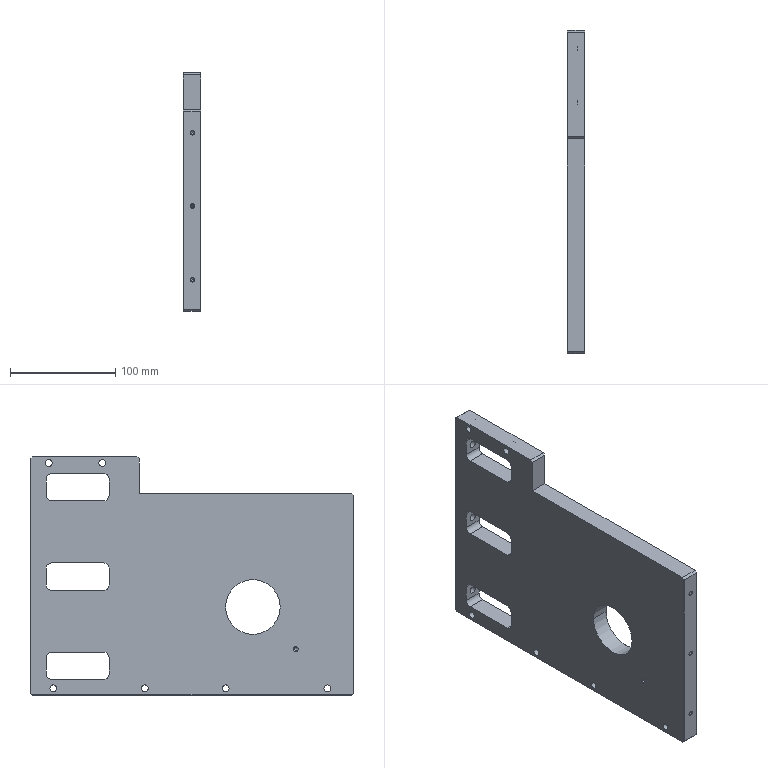Part | NX | 1 solid | 117 faces | box 17 x 308 x 227 mm | volume 943309 mm3 | cylinder 56 | plane 37 | cone 24 | commonest cylinder face diameters 3.3 x12 6.6 x12 10 x12 12 x8 7 x6 11 x4